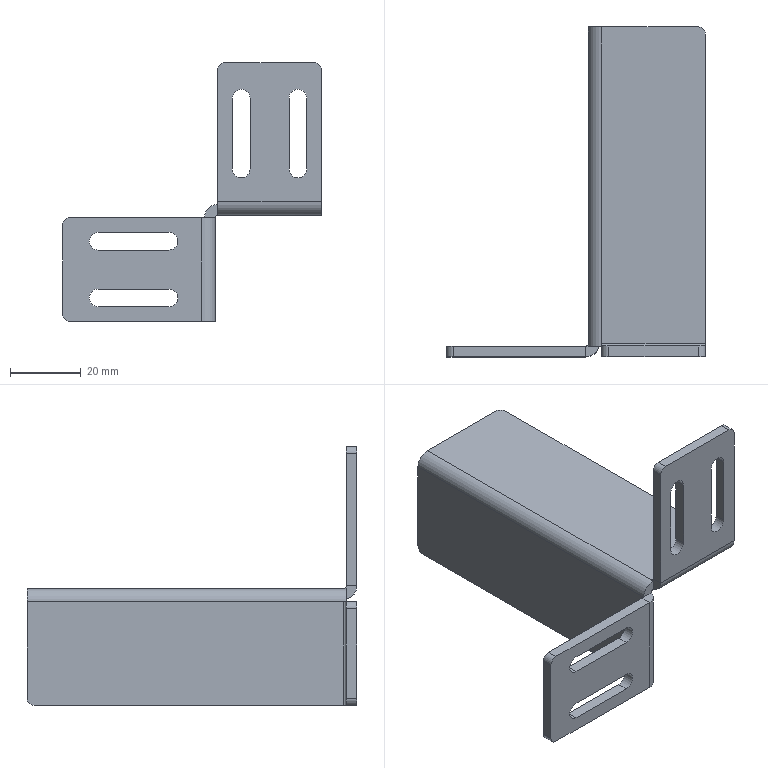Part | STEP file | 护Plate 2 | 1 solid | 58 faces | box 73 x 93 x 73 mm | volume 22681 mm3 | plane 34 | cylinder 24 | commonest cylinder face diameters 5 x12 4 x6 1.473 x3 7.473 x3